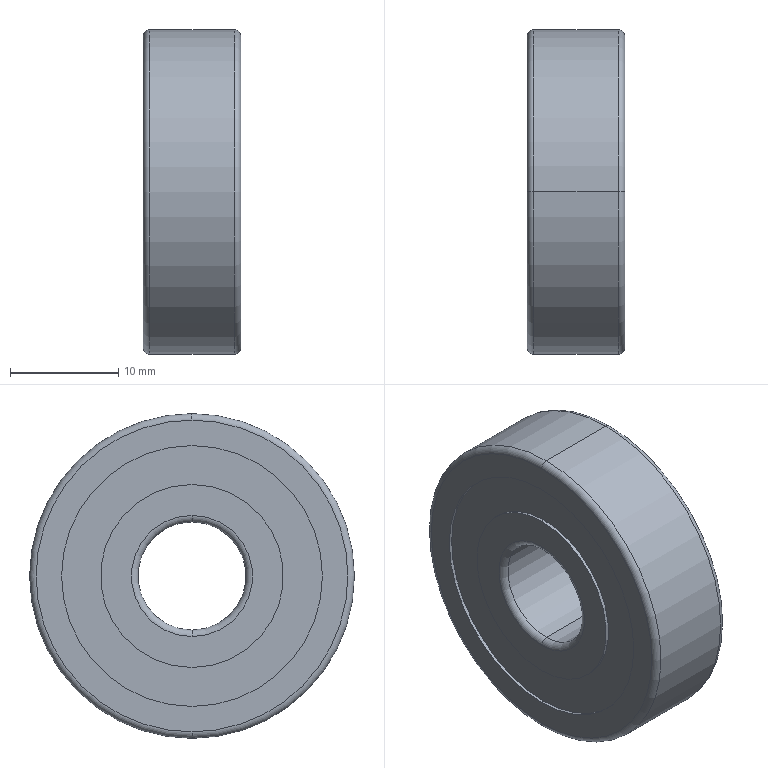Part | STEP file | C-SB6200ZZ-8 | 1 solid | 26 faces | box 9 x 30 x 30 mm | volume 5496 mm3 | cylinder 12 | torus 8 | plane 6 | commonest cylinder face diameters 16.9 x4 24.1 x4 10 x2 30 x2
STEP:
#1=CARTESIAN_POINT('',(0.6,0.,5.));
#2=VERTEX_POINT('',#1);
#3=CARTESIAN_POINT('',(0.6,0.,-5.));
#4=VERTEX_POINT('',#3);
#5=CARTESIAN_POINT('',(0.6,0.,0.));
#6=DIRECTION('',(-1.,0.,0.));
#7=DIRECTION('',(0.,0.,-1.));
#8=AXIS2_PLACEMENT_3D('',#5,#6,#7);
#9=CIRCLE('',#8,5.);
#10=EDGE_CURVE('',#2,#4,#9,.T.);
#11=ORIENTED_EDGE('',*,*,#10,.F.);
#12=CARTESIAN_POINT('',(0.,0.,5.6));
#13=VERTEX_POINT('',#12);
#14=CARTESIAN_POINT('',(0.6,0.,5.6));
#15=DIRECTION('',(0.,1.,0.));
#16=DIRECTION('',(0.,0.,1.));
#17=AXIS2_PLACEMENT_3D('',#14,#15,#16);
#18=CIRCLE('',#17,0.6);
#19=EDGE_CURVE('',#2,#13,#18,.T.);
#20=ORIENTED_EDGE('',*,*,#19,.T.);
#21=CARTESIAN_POINT('',(0.,0.,-5.6));
#22=VERTEX_POINT('',#21);
#23=CARTESIAN_POINT('',(0.,0.,0.));
#24=DIRECTION('',(1.,0.,0.));
#25=DIRECTION('',(0.,0.,-1.));
#26=AXIS2_PLACEMENT_3D('',#23,#24,#25);
#27=CIRCLE('',#26,5.6);
#28=EDGE_CURVE('',#22,#13,#27,.T.);
#29=ORIENTED_EDGE('',*,*,#28,.F.);
#30=CARTESIAN_POINT('',(0.6,0.,-5.6));
#31=DIRECTION('',(0.,-1.,0.));
#32=DIRECTION('',(0.,0.,-1.));
#33=AXIS2_PLACEMENT_3D('',#30,#31,#32);
#34=CIRCLE('',#33,0.6);
#35=EDGE_CURVE('',#4,#22,#34,.T.);
#36=ORIENTED_EDGE('',*,*,#35,.F.);
#37=EDGE_LOOP('',(#11,#20,#29,#36));
#38=FACE_OUTER_BOUND('',#37,.T.);
#39=CARTESIAN_POINT('',(0.6,0.,0.));
#40=DIRECTION('',(1.,0.,0.));
#41=DIRECTION('',(0.,0.,-1.));
#42=AXIS2_PLACEMENT_3D('',#39,#40,#41);
#43=TOROIDAL_SURFACE('',#42,5.6,0.6);
#44=ADVANCED_FACE('',(#38),#43,.T.);
#45=CARTESIAN_POINT('',(8.4,0.,-5.));
#46=VERTEX_POINT('',#45);
#47=CARTESIAN_POINT('',(8.4,0.,5.));
#48=VERTEX_POINT('',#47);
#49=CARTESIAN_POINT('',(8.4,0.,0.));
#50=DIRECTION('',(1.,0.,0.));
#51=DIRECTION('',(0.,0.,1.));
#52=AXIS2_PLACEMENT_3D('',#49,#50,#51);
#53=CIRCLE('',#52,5.);
#54=EDGE_CURVE('',#46,#48,#53,.T.);
#55=ORIENTED_EDGE('',*,*,#54,.F.);
#56=CARTESIAN_POINT('',(9.,0.,-5.6));
#57=VERTEX_POINT('',#56);
#58=CARTESIAN_POINT('',(8.4,0.,-5.6));
#59=DIRECTION('',(0.,1.,0.));
#60=DIRECTION('',(0.,0.,1.));
#61=AXIS2_PLACEMENT_3D('',#58,#59,#60);
#62=CIRCLE('',#61,0.6);
#63=EDGE_CURVE('',#46,#57,#62,.T.);
#64=ORIENTED_EDGE('',*,*,#63,.T.);
#65=CARTESIAN_POINT('',(9.,0.,5.6));
#66=VERTEX_POINT('',#65);
#67=CARTESIAN_POINT('',(9.,0.,0.));
#68=DIRECTION('',(-1.,0.,0.));
#69=DIRECTION('',(0.,0.,1.));
#70=AXIS2_PLACEMENT_3D('',#67,#68,#69);
#71=CIRCLE('',#70,5.6);
#72=EDGE_CURVE('',#66,#57,#71,.T.);
#73=ORIENTED_EDGE('',*,*,#72,.F.);
#74=CARTESIAN_POINT('',(8.4,0.,5.6));
#75=DIRECTION('',(0.,-1.,0.));
#76=DIRECTION('',(0.,0.,-1.));
#77=AXIS2_PLACEMENT_3D('',#74,#75,#76);
#78=CIRCLE('',#77,0.6);
#79=EDGE_CURVE('',#48,#66,#78,.T.);
#80=ORIENTED_EDGE('',*,*,#79,.F.);
#81=EDGE_LOOP('',(#55,#64,#73,#80));
#82=FACE_OUTER_BOUND('',#81,.T.);
#83=CARTESIAN_POINT('',(8.4,0.,0.));
#84=DIRECTION('',(-1.,0.,0.));
#85=DIRECTION('',(0.,0.,1.));
#86=AXIS2_PLACEMENT_3D('',#83,#84,#85);
#87=TOROIDAL_SURFACE('',#86,5.6,0.6);
#88=ADVANCED_FACE('',(#82),#87,.T.);
#89=CARTESIAN_POINT('',(0.,0.,14.4));
#90=VERTEX_POINT('',#89);
#91=CARTESIAN_POINT('',(0.,0.,-14.4));
#92=VERTEX_POINT('',#91);
#93=CARTESIAN_POINT('',(0.,0.,0.));
#94=DIRECTION('',(-1.,0.,0.));
#95=DIRECTION('',(0.,0.,-1.));
#96=AXIS2_PLACEMENT_3D('',#93,#94,#95);
#97=CIRCLE('',#96,14.4);
#98=EDGE_CURVE('',#90,#92,#97,.T.);
#99=ORIENTED_EDGE('',*,*,#98,.F.);
#100=CARTESIAN_POINT('',(0.6,0.,15.));
#101=VERTEX_POINT('',#100);
#102=CARTESIAN_POINT('',(0.6,0.,14.4));
#103=DIRECTION('',(0.,1.,0.));
#104=DIRECTION('',(0.,0.,1.));
#105=AXIS2_PLACEMENT_3D('',#102,#103,#104);
#106=CIRCLE('',#105,0.6);
#107=EDGE_CURVE('',#90,#101,#106,.T.);
#108=ORIENTED_EDGE('',*,*,#107,.T.);
#109=CARTESIAN_POINT('',(0.6,0.,-15.));
#110=VERTEX_POINT('',#109);
#111=CARTESIAN_POINT('',(0.6,0.,0.));
#112=DIRECTION('',(1.,0.,0.));
#113=DIRECTION('',(0.,0.,-1.));
#114=AXIS2_PLACEMENT_3D('',#111,#112,#113);
#115=CIRCLE('',#114,15.);
#116=EDGE_CURVE('',#110,#101,#115,.T.);
#117=ORIENTED_EDGE('',*,*,#116,.F.);
#118=CARTESIAN_POINT('',(0.6,0.,-14.4));
#119=DIRECTION('',(0.,-1.,0.));
#120=DIRECTION('',(0.,0.,-1.));
#121=AXIS2_PLACEMENT_3D('',#118,#119,#120);
#122=CIRCLE('',#121,0.6);
#123=EDGE_CURVE('',#92,#110,#122,.T.);
#124=ORIENTED_EDGE('',*,*,#123,.F.);
#125=EDGE_LOOP('',(#99,#108,#117,#124));
#126=FACE_OUTER_BOUND('',#125,.T.);
#127=CARTESIAN_POINT('',(0.6,0.,0.));
#128=DIRECTION('',(1.,0.,0.));
#129=DIRECTION('',(0.,0.,-1.));
#130=AXIS2_PLACEMENT_3D('',#127,#128,#129);
#131=TOROIDAL_SURFACE('',#130,14.4,0.6);
#132=ADVANCED_FACE('',(#126),#131,.T.);
#133=CARTESIAN_POINT('',(9.,0.,-14.4));
#134=VERTEX_POINT('',#133);
#135=CARTESIAN_POINT('',(9.,0.,14.4));
#136=VERTEX_POINT('',#135);
#137=CARTESIAN_POINT('',(9.,0.,0.));
#138=DIRECTION('',(1.,0.,0.));
#139=DIRECTION('',(0.,0.,1.));
#140=AXIS2_PLACEMENT_3D('',#137,#138,#139);
#141=CIRCLE('',#140,14.4);
#142=EDGE_CURVE('',#134,#136,#141,.T.);
#143=ORIENTED_EDGE('',*,*,#142,.F.);
#144=CARTESIAN_POINT('',(8.4,0.,-15.));
#145=VERTEX_POINT('',#144);
#146=CARTESIAN_POINT('',(8.4,0.,-14.4));
#147=DIRECTION('',(0.,1.,0.));
#148=DIRECTION('',(0.,0.,1.));
#149=AXIS2_PLACEMENT_3D('',#146,#147,#148);
#150=CIRCLE('',#149,0.6);
#151=EDGE_CURVE('',#134,#145,#150,.T.);
#152=ORIENTED_EDGE('',*,*,#151,.T.);
#153=CARTESIAN_POINT('',(8.4,0.,15.));
#154=VERTEX_POINT('',#153);
#155=CARTESIAN_POINT('',(8.4,0.,0.));
#156=DIRECTION('',(-1.,0.,0.));
#157=DIRECTION('',(0.,0.,1.));
#158=AXIS2_PLACEMENT_3D('',#155,#156,#157);
#159=CIRCLE('',#158,15.);
#160=EDGE_CURVE('',#154,#145,#159,.T.);
#161=ORIENTED_EDGE('',*,*,#160,.F.);
#162=CARTESIAN_POINT('',(8.4,0.,14.4));
#163=DIRECTION('',(0.,-1.,0.));
#164=DIRECTION('',(0.,0.,-1.));
#165=AXIS2_PLACEMENT_3D('',#162,#163,#164);
#166=CIRCLE('',#165,0.6);
#167=EDGE_CURVE('',#136,#154,#166,.T.);
#168=ORIENTED_EDGE('',*,*,#167,.F.);
#169=EDGE_LOOP('',(#143,#152,#161,#168));
#170=FACE_OUTER_BOUND('',#169,.T.);
#171=CARTESIAN_POINT('',(8.4,0.,0.));
#172=DIRECTION('',(-1.,0.,0.));
#173=DIRECTION('',(0.,0.,1.));
#174=AXIS2_PLACEMENT_3D('',#171,#172,#173);
#175=TOROIDAL_SURFACE('',#174,14.4,0.6);
#176=ADVANCED_FACE('',(#170),#175,.T.);
#177=ORIENTED_EDGE('',*,*,#160,.T.);
#178=CARTESIAN_POINT('',(0.,0.,-15.));
#179=DIRECTION('',(-1.,0.,0.));
#180=VECTOR('',#179,1000.);
#181=LINE('',#178,#180);
#182=EDGE_CURVE('',#145,#110,#181,.T.);
#183=ORIENTED_EDGE('',*,*,#182,.T.);
#184=ORIENTED_EDGE('',*,*,#116,.T.);
#185=CARTESIAN_POINT('',(0.,0.,15.));
#186=DIRECTION('',(-1.,0.,0.));
#187=VECTOR('',#186,1000.);
#188=LINE('',#185,#187);
#189=EDGE_CURVE('',#154,#101,#188,.T.);
#190=ORIENTED_EDGE('',*,*,#189,.F.);
#191=EDGE_LOOP('',(#177,#183,#184,#190));
#192=FACE_OUTER_BOUND('',#191,.T.);
#193=CARTESIAN_POINT('',(0.,0.,0.));
#194=DIRECTION('',(-1.,0.,0.));
#195=DIRECTION('',(0.,0.,1.));
#196=AXIS2_PLACEMENT_3D('',#193,#194,#195);
#197=CYLINDRICAL_SURFACE('',#196,15.);
#198=ADVANCED_FACE('',(#192),#197,.T.);
#199=CARTESIAN_POINT('',(9.,0.,-12.05));
#200=VERTEX_POINT('',#199);
#201=CARTESIAN_POINT('',(9.,0.,12.05));
#202=VERTEX_POINT('',#201);
#203=CARTESIAN_POINT('',(9.,0.,0.));
#204=DIRECTION('',(-1.,0.,0.));
#205=DIRECTION('',(0.,0.,1.));
#206=AXIS2_PLACEMENT_3D('',#203,#204,#205);
#207=CIRCLE('',#206,12.05);
#208=EDGE_CURVE('',#200,#202,#207,.T.);
#209=ORIENTED_EDGE('',*,*,#208,.F.);
#210=CARTESIAN_POINT('',(8.7,0.,-12.05));
#211=VERTEX_POINT('',#210);
#212=CARTESIAN_POINT('',(0.,0.,-12.05));
#213=DIRECTION('',(-1.,0.,0.));
#214=VECTOR('',#213,1000.);
#215=LINE('',#212,#214);
#216=EDGE_CURVE('',#200,#211,#215,.T.);
#217=ORIENTED_EDGE('',*,*,#216,.T.);
#218=CARTESIAN_POINT('',(8.7,0.,12.05));
#219=VERTEX_POINT('',#218);
#220=CARTESIAN_POINT('',(8.7,0.,0.));
#221=DIRECTION('',(-1.,0.,0.));
#222=DIRECTION('',(0.,0.,1.));
#223=AXIS2_PLACEMENT_3D('',#220,#221,#222);
#224=CIRCLE('',#223,12.05);
#225=EDGE_CURVE('',#211,#219,#224,.T.);
#226=ORIENTED_EDGE('',*,*,#225,.T.);
#227=CARTESIAN_POINT('',(0.,0.,12.05));
#228=DIRECTION('',(-1.,0.,0.));
#229=VECTOR('',#228,1000.);
#230=LINE('',#227,#229);
#231=EDGE_CURVE('',#202,#219,#230,.T.);
#232=ORIENTED_EDGE('',*,*,#231,.F.);
#233=EDGE_LOOP('',(#209,#217,#226,#232));
#234=FACE_OUTER_BOUND('',#233,.T.);
#235=CARTESIAN_POINT('',(0.,0.,0.));
#236=DIRECTION('',(-1.,0.,0.));
#237=DIRECTION('',(0.,0.,1.));
#238=AXIS2_PLACEMENT_3D('',#235,#236,#237);
#239=CYLINDRICAL_SURFACE('',#238,12.05);
#240=ADVANCED_FACE('',(#234),#239,.F.);
#241=CARTESIAN_POINT('',(9.,0.,8.45));
#242=VERTEX_POINT('',#241);
#243=CARTESIAN_POINT('',(9.,0.,-8.45));
#244=VERTEX_POINT('',#243);
#245=CARTESIAN_POINT('',(9.,0.,0.));
#246=DIRECTION('',(-1.,0.,0.));
#247=DIRECTION('',(0.,0.,1.));
#248=AXIS2_PLACEMENT_3D('',#245,#246,#247);
#249=CIRCLE('',#248,8.45);
#250=EDGE_CURVE('',#242,#244,#249,.T.);
#251=ORIENTED_EDGE('',*,*,#250,.T.);
#252=CARTESIAN_POINT('',(8.7,0.,-8.45));
#253=VERTEX_POINT('',#252);
#254=CARTESIAN_POINT('',(0.,0.,-8.45));
#255=DIRECTION('',(-1.,0.,0.));
#256=VECTOR('',#255,1000.);
#257=LINE('',#254,#256);
#258=EDGE_CURVE('',#244,#253,#257,.T.);
#259=ORIENTED_EDGE('',*,*,#258,.T.);
#260=CARTESIAN_POINT('',(8.7,0.,8.45));
#261=VERTEX_POINT('',#260);
#262=CARTESIAN_POINT('',(8.7,0.,0.));
#263=DIRECTION('',(-1.,0.,0.));
#264=DIRECTION('',(0.,0.,1.));
#265=AXIS2_PLACEMENT_3D('',#262,#263,#264);
#266=CIRCLE('',#265,8.45);
#267=EDGE_CURVE('',#261,#253,#266,.T.);
#268=ORIENTED_EDGE('',*,*,#267,.F.);
#269=CARTESIAN_POINT('',(0.,0.,8.45));
#270=DIRECTION('',(-1.,0.,0.));
#271=VECTOR('',#270,1000.);
#272=LINE('',#269,#271);
#273=EDGE_CURVE('',#242,#261,#272,.T.);
#274=ORIENTED_EDGE('',*,*,#273,.F.);
#275=EDGE_LOOP('',(#251,#259,#268,#274));
#276=FACE_OUTER_BOUND('',#275,.T.);
#277=CARTESIAN_POINT('',(0.,0.,0.));
#278=DIRECTION('',(-1.,0.,0.));
#279=DIRECTION('',(0.,0.,1.));
#280=AXIS2_PLACEMENT_3D('',#277,#278,#279);
#281=CYLINDRICAL_SURFACE('',#280,8.45);
#282=ADVANCED_FACE('',(#276),#281,.T.);
#283=CARTESIAN_POINT('',(8.4,0.,0.));
#284=DIRECTION('',(1.,0.,0.));
#285=DIRECTION('',(0.,0.,1.));
#286=AXIS2_PLACEMENT_3D('',#283,#284,#285);
#287=CIRCLE('',#286,5.);
#288=EDGE_CURVE('',#48,#46,#287,.T.);
#289=ORIENTED_EDGE('',*,*,#288,.T.);
#290=CARTESIAN_POINT('',(0.,0.,-5.));
#291=DIRECTION('',(-1.,0.,0.));
#292=VECTOR('',#291,1000.);
#293=LINE('',#290,#292);
#294=EDGE_CURVE('',#46,#4,#293,.T.);
#295=ORIENTED_EDGE('',*,*,#294,.T.);
#296=CARTESIAN_POINT('',(0.6,0.,0.));
#297=DIRECTION('',(-1.,0.,0.));
#298=DIRECTION('',(0.,0.,-1.));
#299=AXIS2_PLACEMENT_3D('',#296,#297,#298);
#300=CIRCLE('',#299,5.);
#301=EDGE_CURVE('',#4,#2,#300,.T.);
#302=ORIENTED_EDGE('',*,*,#301,.T.);
#303=CARTESIAN_POINT('',(0.,0.,5.));
#304=DIRECTION('',(-1.,0.,0.));
#305=VECTOR('',#304,1000.);
#306=LINE('',#303,#305);
#307=EDGE_CURVE('',#48,#2,#306,.T.);
#308=ORIENTED_EDGE('',*,*,#307,.F.);
#309=EDGE_LOOP('',(#289,#295,#302,#308));
#310=FACE_OUTER_BOUND('',#309,.T.);
#311=CARTESIAN_POINT('',(0.,0.,0.));
#312=DIRECTION('',(-1.,0.,0.));
#313=DIRECTION('',(0.,0.,1.));
#314=AXIS2_PLACEMENT_3D('',#311,#312,#313);
#315=CYLINDRICAL_SURFACE('',#314,5.);
#316=ADVANCED_FACE('',(#310),#315,.F.);
#317=CARTESIAN_POINT('',(0.3,0.,8.45));
#318=VERTEX_POINT('',#317);
#319=CARTESIAN_POINT('',(0.3,0.,-8.45));
#320=VERTEX_POINT('',#319);
#321=CARTESIAN_POINT('',(0.3,0.,0.));
#322=DIRECTION('',(-1.,0.,0.));
#323=DIRECTION('',(0.,0.,1.));
#324=AXIS2_PLACEMENT_3D('',#321,#322,#323);
#325=CIRCLE('',#324,8.45);
#326=EDGE_CURVE('',#318,#320,#325,.T.);
#327=ORIENTED_EDGE('',*,*,#326,.T.);
#328=CARTESIAN_POINT('',(0.,0.,-8.45));
#329=VERTEX_POINT('',#328);
#330=CARTESIAN_POINT('',(0.,0.,-8.45));
#331=DIRECTION('',(-1.,0.,0.));
#332=VECTOR('',#331,1000.);
#333=LINE('',#330,#332);
#334=EDGE_CURVE('',#320,#329,#333,.T.);
#335=ORIENTED_EDGE('',*,*,#334,.T.);
#336=CARTESIAN_POINT('',(0.,0.,8.45));
#337=VERTEX_POINT('',#336);
#338=CARTESIAN_POINT('',(0.,0.,0.));
#339=DIRECTION('',(-1.,0.,0.));
#340=DIRECTION('',(0.,0.,1.));
#341=AXIS2_PLACEMENT_3D('',#338,#339,#340);
#342=CIRCLE('',#341,8.45);
#343=EDGE_CURVE('',#337,#329,#342,.T.);
#344=ORIENTED_EDGE('',*,*,#343,.F.);
#345=CARTESIAN_POINT('',(0.,0.,8.45));
#346=DIRECTION('',(-1.,0.,0.));
#347=VECTOR('',#346,1000.);
#348=LINE('',#345,#347);
#349=EDGE_CURVE('',#318,#337,#348,.T.);
#350=ORIENTED_EDGE('',*,*,#349,.F.);
#351=EDGE_LOOP('',(#327,#335,#344,#350));
#352=FACE_OUTER_BOUND('',#351,.T.);
#353=CARTESIAN_POINT('',(0.,0.,0.));
#354=DIRECTION('',(-1.,0.,0.));
#355=DIRECTION('',(0.,0.,1.));
#356=AXIS2_PLACEMENT_3D('',#353,#354,#355);
#357=CYLINDRICAL_SURFACE('',#356,8.45);
#358=ADVANCED_FACE('',(#352),#357,.T.);
#359=CARTESIAN_POINT('',(0.3,0.,-12.05));
#360=VERTEX_POINT('',#359);
#361=CARTESIAN_POINT('',(0.3,0.,12.05));
#362=VERTEX_POINT('',#361);
#363=CARTESIAN_POINT('',(0.3,0.,0.));
#364=DIRECTION('',(-1.,0.,0.));
#365=DIRECTION('',(0.,0.,1.));
#366=AXIS2_PLACEMENT_3D('',#363,#364,#365);
#367=CIRCLE('',#366,12.05);
#368=EDGE_CURVE('',#360,#362,#367,.T.);
#369=ORIENTED_EDGE('',*,*,#368,.F.);
#370=CARTESIAN_POINT('',(0.,0.,-12.05));
#371=VERTEX_POINT('',#370);
#372=CARTESIAN_POINT('',(0.,0.,-12.05));
#373=DIRECTION('',(-1.,0.,0.));
#374=VECTOR('',#373,1000.);
#375=LINE('',#372,#374);
#376=EDGE_CURVE('',#360,#371,#375,.T.);
#377=ORIENTED_EDGE('',*,*,#376,.T.);
#378=CARTESIAN_POINT('',(0.,0.,12.05));
#379=VERTEX_POINT('',#378);
#380=CARTESIAN_POINT('',(0.,0.,0.));
#381=DIRECTION('',(-1.,0.,0.));
#382=DIRECTION('',(0.,0.,1.));
#383=AXIS2_PLACEMENT_3D('',#380,#381,#382);
#384=CIRCLE('',#383,12.05);
#385=EDGE_CURVE('',#371,#379,#384,.T.);
#386=ORIENTED_EDGE('',*,*,#385,.T.);
#387=CARTESIAN_POINT('',(0.,0.,12.05));
#388=DIRECTION('',(-1.,0.,0.));
#389=VECTOR('',#388,1000.);
#390=LINE('',#387,#389);
#391=EDGE_CURVE('',#362,#379,#390,.T.);
#392=ORIENTED_EDGE('',*,*,#391,.F.);
#393=EDGE_LOOP('',(#369,#377,#386,#392));
#394=FACE_OUTER_BOUND('',#393,.T.);
#395=CARTESIAN_POINT('',(0.,0.,0.));
#396=DIRECTION('',(-1.,0.,0.));
#397=DIRECTION('',(0.,0.,1.));
#398=AXIS2_PLACEMENT_3D('',#395,#396,#397);
#399=CYLINDRICAL_SURFACE('',#398,12.05);
#400=ADVANCED_FACE('',(#394),#399,.F.);
#401=CARTESIAN_POINT('',(0.,0.,0.));
#402=DIRECTION('',(-1.,0.,0.));
#403=DIRECTION('',(0.,0.,-1.));
#404=AXIS2_PLACEMENT_3D('',#401,#402,#403);
#405=CIRCLE('',#404,14.4);
#406=EDGE_CURVE('',#92,#90,#405,.T.);
#407=ORIENTED_EDGE('',*,*,#406,.T.);
#408=ORIENTED_EDGE('',*,*,#98,.T.);
#409=EDGE_LOOP('',(#407,#408));
#410=FACE_OUTER_BOUND('',#409,.T.);
#411=CARTESIAN_POINT('',(0.,0.,0.));
#412=DIRECTION('',(-1.,0.,0.));
#413=DIRECTION('',(0.,0.,1.));
#414=AXIS2_PLACEMENT_3D('',#411,#412,#413);
#415=CIRCLE('',#414,12.05);
#416=EDGE_CURVE('',#379,#371,#415,.T.);
#417=ORIENTED_EDGE('',*,*,#416,.F.);
#418=ORIENTED_EDGE('',*,*,#385,.F.);
#419=EDGE_LOOP('',(#417,#418));
#420=FACE_BOUND('',#419,.T.);
#421=CARTESIAN_POINT('',(0.,15.,0.));
#422=DIRECTION('',(1.,0.,0.));
#423=DIRECTION('',(0.,0.,-1.));
#424=AXIS2_PLACEMENT_3D('',#421,#422,#423);
#425=PLANE('',#424);
#426=ADVANCED_FACE('',(#410,#420),#425,.F.);
#427=ORIENTED_EDGE('',*,*,#376,.F.);
#428=CARTESIAN_POINT('',(0.3,0.,0.));
#429=DIRECTION('',(-1.,0.,0.));
#430=DIRECTION('',(0.,0.,1.));
#431=AXIS2_PLACEMENT_3D('',#428,#429,#430);
#432=CIRCLE('',#431,12.05);
#433=EDGE_CURVE('',#362,#360,#432,.T.);
#434=ORIENTED_EDGE('',*,*,#433,.F.);
#435=ORIENTED_EDGE('',*,*,#391,.T.);
#436=ORIENTED_EDGE('',*,*,#416,.T.);
#437=EDGE_LOOP('',(#427,#434,#435,#436));
#438=FACE_OUTER_BOUND('',#437,.T.);
#439=CARTESIAN_POINT('',(0.,0.,0.));
#440=DIRECTION('',(-1.,0.,0.));
#441=DIRECTION('',(0.,0.,1.));
#442=AXIS2_PLACEMENT_3D('',#439,#440,#441);
#443=CYLINDRICAL_SURFACE('',#442,12.05);
#444=ADVANCED_FACE('',(#438),#443,.F.);
#445=ORIENTED_EDGE('',*,*,#326,.F.);
#446=CARTESIAN_POINT('',(0.3,0.,0.));
#447=DIRECTION('',(-1.,0.,0.));
#448=DIRECTION('',(0.,0.,1.));
#449=AXIS2_PLACEMENT_3D('',#446,#447,#448);
#450=CIRCLE('',#449,8.45);
#451=EDGE_CURVE('',#320,#318,#450,.T.);
#452=ORIENTED_EDGE('',*,*,#451,.F.);
#453=EDGE_LOOP('',(#445,#452));
#454=FACE_BOUND('',#453,.T.);
#455=ORIENTED_EDGE('',*,*,#433,.T.);
#456=ORIENTED_EDGE('',*,*,#368,.T.);
#457=EDGE_LOOP('',(#455,#456));
#458=FACE_OUTER_BOUND('',#457,.T.);
#459=CARTESIAN_POINT('',(0.3,12.05,0.));
#460=DIRECTION('',(1.,0.,0.));
#461=DIRECTION('',(0.,0.,-1.));
#462=AXIS2_PLACEMENT_3D('',#459,#460,#461);
#463=PLANE('',#462);
#464=ADVANCED_FACE('',(#454,#458),#463,.F.);
#465=ORIENTED_EDGE('',*,*,#334,.F.);
#466=ORIENTED_EDGE('',*,*,#451,.T.);
#467=ORIENTED_EDGE('',*,*,#349,.T.);
#468=CARTESIAN_POINT('',(0.,0.,0.));
#469=DIRECTION('',(-1.,0.,0.));
#470=DIRECTION('',(0.,0.,1.));
#471=AXIS2_PLACEMENT_3D('',#468,#469,#470);
#472=CIRCLE('',#471,8.45);
#473=EDGE_CURVE('',#329,#337,#472,.T.);
#474=ORIENTED_EDGE('',*,*,#473,.F.);
#475=EDGE_LOOP('',(#465,#466,#467,#474));
#476=FACE_OUTER_BOUND('',#475,.T.);
#477=CARTESIAN_POINT('',(0.,0.,0.));
#478=DIRECTION('',(-1.,0.,0.));
#479=DIRECTION('',(0.,0.,1.));
#480=AXIS2_PLACEMENT_3D('',#477,#478,#479);
#481=CYLINDRICAL_SURFACE('',#480,8.45);
#482=ADVANCED_FACE('',(#476),#481,.T.);
#483=ORIENTED_EDGE('',*,*,#28,.T.);
#484=CARTESIAN_POINT('',(0.,0.,0.));
#485=DIRECTION('',(1.,0.,0.));
#486=DIRECTION('',(0.,0.,-1.));
#487=AXIS2_PLACEMENT_3D('',#484,#485,#486);
#488=CIRCLE('',#487,5.6);
#489=EDGE_CURVE('',#13,#22,#488,.T.);
#490=ORIENTED_EDGE('',*,*,#489,.T.);
#491=EDGE_LOOP('',(#483,#490));
#492=FACE_BOUND('',#491,.T.);
#493=ORIENTED_EDGE('',*,*,#343,.T.);
#494=ORIENTED_EDGE('',*,*,#473,.T.);
#495=EDGE_LOOP('',(#493,#494));
#496=FACE_OUTER_BOUND('',#495,.T.);
#497=CARTESIAN_POINT('',(0.,8.45,0.));
#498=DIRECTION('',(1.,0.,0.));
#499=DIRECTION('',(0.,0.,-1.));
#500=AXIS2_PLACEMENT_3D('',#497,#498,#499);
#501=PLANE('',#500);
#502=ADVANCED_FACE('',(#492,#496),#501,.F.);
#503=ORIENTED_EDGE('',*,*,#294,.F.);
#504=ORIENTED_EDGE('',*,*,#54,.T.);
#505=ORIENTED_EDGE('',*,*,#307,.T.);
#506=ORIENTED_EDGE('',*,*,#10,.T.);
#507=EDGE_LOOP('',(#503,#504,#505,#506));
#508=FACE_OUTER_BOUND('',#507,.T.);
#509=CARTESIAN_POINT('',(0.,0.,0.));
#510=DIRECTION('',(-1.,0.,0.));
#511=DIRECTION('',(0.,0.,1.));
#512=AXIS2_PLACEMENT_3D('',#509,#510,#511);
#513=CYLINDRICAL_SURFACE('',#512,5.);
#514=ADVANCED_FACE('',(#508),#513,.F.);
#515=ORIENTED_EDGE('',*,*,#72,.T.);
#516=CARTESIAN_POINT('',(9.,0.,0.));
#517=DIRECTION('',(-1.,0.,0.));
#518=DIRECTION('',(0.,0.,1.));
#519=AXIS2_PLACEMENT_3D('',#516,#517,#518);
#520=CIRCLE('',#519,5.6);
#521=EDGE_CURVE('',#57,#66,#520,.T.);
#522=ORIENTED_EDGE('',*,*,#521,.T.);
#523=EDGE_LOOP('',(#515,#522));
#524=FACE_BOUND('',#523,.T.);
#525=ORIENTED_EDGE('',*,*,#250,.F.);
#526=CARTESIAN_POINT('',(9.,0.,0.));
#527=DIRECTION('',(-1.,0.,0.));
#528=DIRECTION('',(0.,0.,1.));
#529=AXIS2_PLACEMENT_3D('',#526,#527,#528);
#530=CIRCLE('',#529,8.45);
#531=EDGE_CURVE('',#244,#242,#530,.T.);
#532=ORIENTED_EDGE('',*,*,#531,.F.);
#533=EDGE_LOOP('',(#525,#532));
#534=FACE_OUTER_BOUND('',#533,.T.);
#535=CARTESIAN_POINT('',(9.,8.45,0.));
#536=DIRECTION('',(-1.,0.,0.));
#537=DIRECTION('',(0.,0.,1.));
#538=AXIS2_PLACEMENT_3D('',#535,#536,#537);
#539=PLANE('',#538);
#540=ADVANCED_FACE('',(#524,#534),#539,.F.);
#541=ORIENTED_EDGE('',*,*,#258,.F.);
#542=ORIENTED_EDGE('',*,*,#531,.T.);
#543=ORIENTED_EDGE('',*,*,#273,.T.);
#544=CARTESIAN_POINT('',(8.7,0.,0.));
#545=DIRECTION('',(-1.,0.,0.));
#546=DIRECTION('',(0.,0.,1.));
#547=AXIS2_PLACEMENT_3D('',#544,#545,#546);
#548=CIRCLE('',#547,8.45);
#549=EDGE_CURVE('',#253,#261,#548,.T.);
#550=ORIENTED_EDGE('',*,*,#549,.F.);
#551=EDGE_LOOP('',(#541,#542,#543,#550));
#552=FACE_OUTER_BOUND('',#551,.T.);
#553=CARTESIAN_POINT('',(0.,0.,0.));
#554=DIRECTION('',(-1.,0.,0.));
#555=DIRECTION('',(0.,0.,1.));
#556=AXIS2_PLACEMENT_3D('',#553,#554,#555);
#557=CYLINDRICAL_SURFACE('',#556,8.45);
#558=ADVANCED_FACE('',(#552),#557,.T.);
#559=CARTESIAN_POINT('',(8.7,0.,0.));
#560=DIRECTION('',(-1.,0.,0.));
#561=DIRECTION('',(0.,0.,1.));
#562=AXIS2_PLACEMENT_3D('',#559,#560,#561);
#563=CIRCLE('',#562,12.05);
#564=EDGE_CURVE('',#219,#211,#563,.T.);
#565=ORIENTED_EDGE('',*,*,#564,.F.);
#566=ORIENTED_EDGE('',*,*,#225,.F.);
#567=EDGE_LOOP('',(#565,#566));
#568=FACE_OUTER_BOUND('',#567,.T.);
#569=ORIENTED_EDGE('',*,*,#267,.T.);
#570=ORIENTED_EDGE('',*,*,#549,.T.);
#571=EDGE_LOOP('',(#569,#570));
#572=FACE_BOUND('',#571,.T.);
#573=CARTESIAN_POINT('',(8.7,12.05,0.));
#574=DIRECTION('',(-1.,0.,0.));
#575=DIRECTION('',(0.,0.,1.));
#576=AXIS2_PLACEMENT_3D('',#573,#574,#575);
#577=PLANE('',#576);
#578=ADVANCED_FACE('',(#568,#572),#577,.F.);
#579=ORIENTED_EDGE('',*,*,#216,.F.);
#580=CARTESIAN_POINT('',(9.,0.,0.));
#581=DIRECTION('',(-1.,0.,0.));
#582=DIRECTION('',(0.,0.,1.));
#583=AXIS2_PLACEMENT_3D('',#580,#581,#582);
#584=CIRCLE('',#583,12.05);
#585=EDGE_CURVE('',#202,#200,#584,.T.);
#586=ORIENTED_EDGE('',*,*,#585,.F.);
#587=ORIENTED_EDGE('',*,*,#231,.T.);
#588=ORIENTED_EDGE('',*,*,#564,.T.);
#589=EDGE_LOOP('',(#579,#586,#587,#588));
#590=FACE_OUTER_BOUND('',#589,.T.);
#591=CARTESIAN_POINT('',(0.,0.,0.));
#592=DIRECTION('',(-1.,0.,0.));
#593=DIRECTION('',(0.,0.,1.));
#594=AXIS2_PLACEMENT_3D('',#591,#592,#593);
#595=CYLINDRICAL_SURFACE('',#594,12.05);
#596=ADVANCED_FACE('',(#590),#595,.F.);
#597=CARTESIAN_POINT('',(9.,0.,0.));
#598=DIRECTION('',(1.,0.,0.));
#599=DIRECTION('',(0.,0.,1.));
#600=AXIS2_PLACEMENT_3D('',#597,#598,#599);
#601=CIRCLE('',#600,14.4);
#602=EDGE_CURVE('',#136,#134,#601,.T.);
#603=ORIENTED_EDGE('',*,*,#602,.T.);
#604=ORIENTED_EDGE('',*,*,#142,.T.);
#605=EDGE_LOOP('',(#603,#604));
#606=FACE_OUTER_BOUND('',#605,.T.);
#607=ORIENTED_EDGE('',*,*,#585,.T.);
#608=ORIENTED_EDGE('',*,*,#208,.T.);
#609=EDGE_LOOP('',(#607,#608));
#610=FACE_BOUND('',#609,.T.);
#611=CARTESIAN_POINT('',(9.,15.,0.));
#612=DIRECTION('',(-1.,0.,0.));
#613=DIRECTION('',(0.,0.,1.));
#614=AXIS2_PLACEMENT_3D('',#611,#612,#613);
#615=PLANE('',#614);
#616=ADVANCED_FACE('',(#606,#610),#615,.F.);
#617=ORIENTED_EDGE('',*,*,#182,.F.);
#618=CARTESIAN_POINT('',(8.4,0.,0.));
#619=DIRECTION('',(-1.,0.,0.));
#620=DIRECTION('',(0.,0.,1.));
#621=AXIS2_PLACEMENT_3D('',#618,#619,#620);
#622=CIRCLE('',#621,15.);
#623=EDGE_CURVE('',#145,#154,#622,.T.);
#624=ORIENTED_EDGE('',*,*,#623,.T.);
#625=ORIENTED_EDGE('',*,*,#189,.T.);
#626=CARTESIAN_POINT('',(0.6,0.,0.));
#627=DIRECTION('',(1.,0.,0.));
#628=DIRECTION('',(0.,0.,-1.));
#629=AXIS2_PLACEMENT_3D('',#626,#627,#628);
#630=CIRCLE('',#629,15.);
#631=EDGE_CURVE('',#101,#110,#630,.T.);
#632=ORIENTED_EDGE('',*,*,#631,.T.);
#633=EDGE_LOOP('',(#617,#624,#625,#632));
#634=FACE_OUTER_BOUND('',#633,.T.);
#635=CARTESIAN_POINT('',(0.,0.,0.));
#636=DIRECTION('',(-1.,0.,0.));
#637=DIRECTION('',(0.,0.,1.));
#638=AXIS2_PLACEMENT_3D('',#635,#636,#637);
#639=CYLINDRICAL_SURFACE('',#638,15.);
#640=ADVANCED_FACE('',(#634),#639,.T.);
#641=ORIENTED_EDGE('',*,*,#151,.F.);
#642=ORIENTED_EDGE('',*,*,#602,.F.);
#643=ORIENTED_EDGE('',*,*,#167,.T.);
#644=ORIENTED_EDGE('',*,*,#623,.F.);
#645=EDGE_LOOP('',(#641,#642,#643,#644));
#646=FACE_OUTER_BOUND('',#645,.T.);
#647=CARTESIAN_POINT('',(8.4,0.,0.));
#648=DIRECTION('',(-1.,0.,0.));
#649=DIRECTION('',(0.,0.,1.));
#650=AXIS2_PLACEMENT_3D('',#647,#648,#649);
#651=TOROIDAL_SURFACE('',#650,14.4,0.6);
#652=ADVANCED_FACE('',(#646),#651,.T.);
#653=ORIENTED_EDGE('',*,*,#107,.F.);
#654=ORIENTED_EDGE('',*,*,#406,.F.);
#655=ORIENTED_EDGE('',*,*,#123,.T.);
#656=ORIENTED_EDGE('',*,*,#631,.F.);
#657=EDGE_LOOP('',(#653,#654,#655,#656));
#658=FACE_OUTER_BOUND('',#657,.T.);
#659=CARTESIAN_POINT('',(0.6,0.,0.));
#660=DIRECTION('',(1.,0.,0.));
#661=DIRECTION('',(0.,0.,-1.));
#662=AXIS2_PLACEMENT_3D('',#659,#660,#661);
#663=TOROIDAL_SURFACE('',#662,14.4,0.6);
#664=ADVANCED_FACE('',(#658),#663,.T.);
#665=ORIENTED_EDGE('',*,*,#63,.F.);
#666=ORIENTED_EDGE('',*,*,#288,.F.);
#667=ORIENTED_EDGE('',*,*,#79,.T.);
#668=ORIENTED_EDGE('',*,*,#521,.F.);
#669=EDGE_LOOP('',(#665,#666,#667,#668));
#670=FACE_OUTER_BOUND('',#669,.T.);
#671=CARTESIAN_POINT('',(8.4,0.,0.));
#672=DIRECTION('',(-1.,0.,0.));
#673=DIRECTION('',(0.,0.,1.));
#674=AXIS2_PLACEMENT_3D('',#671,#672,#673);
#675=TOROIDAL_SURFACE('',#674,5.6,0.6);
#676=ADVANCED_FACE('',(#670),#675,.T.);
#677=ORIENTED_EDGE('',*,*,#19,.F.);
#678=ORIENTED_EDGE('',*,*,#301,.F.);
#679=ORIENTED_EDGE('',*,*,#35,.T.);
#680=ORIENTED_EDGE('',*,*,#489,.F.);
#681=EDGE_LOOP('',(#677,#678,#679,#680));
#682=FACE_OUTER_BOUND('',#681,.T.);
#683=CARTESIAN_POINT('',(0.6,0.,0.));
#684=DIRECTION('',(1.,0.,0.));
#685=DIRECTION('',(0.,0.,-1.));
#686=AXIS2_PLACEMENT_3D('',#683,#684,#685);
#687=TOROIDAL_SURFACE('',#686,5.6,0.6);
#688=ADVANCED_FACE('',(#682),#687,.T.);
#689=CLOSED_SHELL('',(#44,#88,#132,#176,#198,#240,#282,#316,#358,#400,#426,#444,#464,#482,#502,#514,#540,#558,#578,#596,#616,#640,#652,#664,#676,#688));
#690=MANIFOLD_SOLID_BREP('',#689);
#691=CARTESIAN_POINT('',(0.,0.,0.));
#692=DIRECTION('',(0.,0.,1.));
#693=DIRECTION('',(1.,0.,0.));
#694=AXIS2_PLACEMENT_3D('',#691,#692,#693);
#695=(LENGTH_UNIT()NAMED_UNIT(*)SI_UNIT(.MILLI.,.METRE.));
#696=UNCERTAINTY_MEASURE_WITH_UNIT(LENGTH_MEASURE(0.00001),#695,'','');
#697=(NAMED_UNIT(*)PLANE_ANGLE_UNIT()SI_UNIT($,.RADIAN.));
#698=(NAMED_UNIT(*)SI_UNIT($,.STERADIAN.)SOLID_ANGLE_UNIT());
#699=(GEOMETRIC_REPRESENTATION_CONTEXT(3)GLOBAL_UNCERTAINTY_ASSIGNED_CONTEXT((#696))GLOBAL_UNIT_ASSIGNED_CONTEXT((#695,#697,#698))REPRESENTATION_CONTEXT('',''));
#700=ADVANCED_BREP_SHAPE_REPRESENTATION('',(#690,#694),#699);